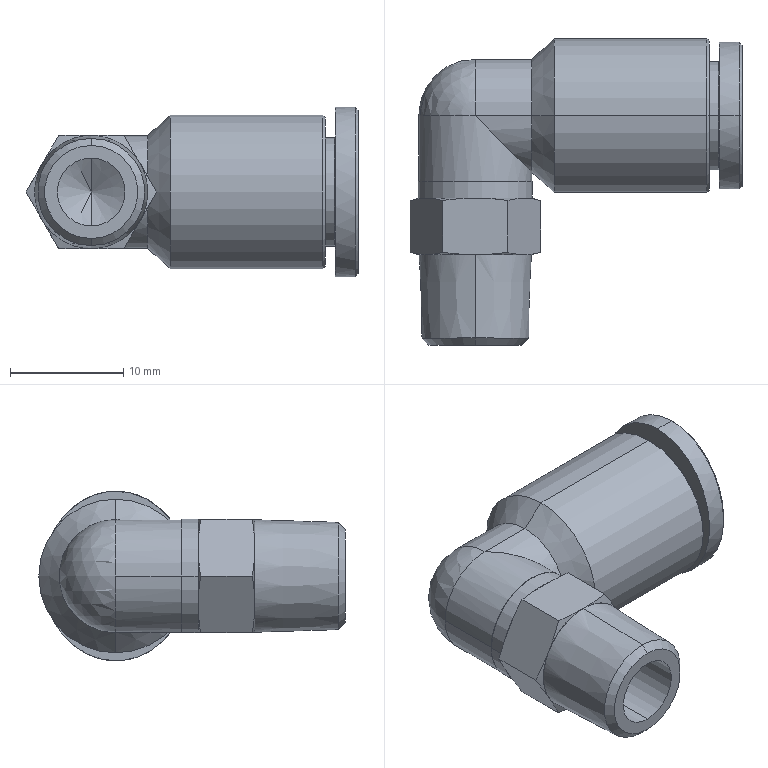Part | STEP file | L-type fitting PL8-01 | 1 solid | 56 faces | box 29.374 x 27.1 x 15 mm | volume 3387 mm3 | cone 22 | cylinder 15 | plane 14 | spline 4 | sphere 1 | commonest cylinder face diameters 10 x5 6 x2 8 x2 9.6 x2 10.1 x2 13.6 x2